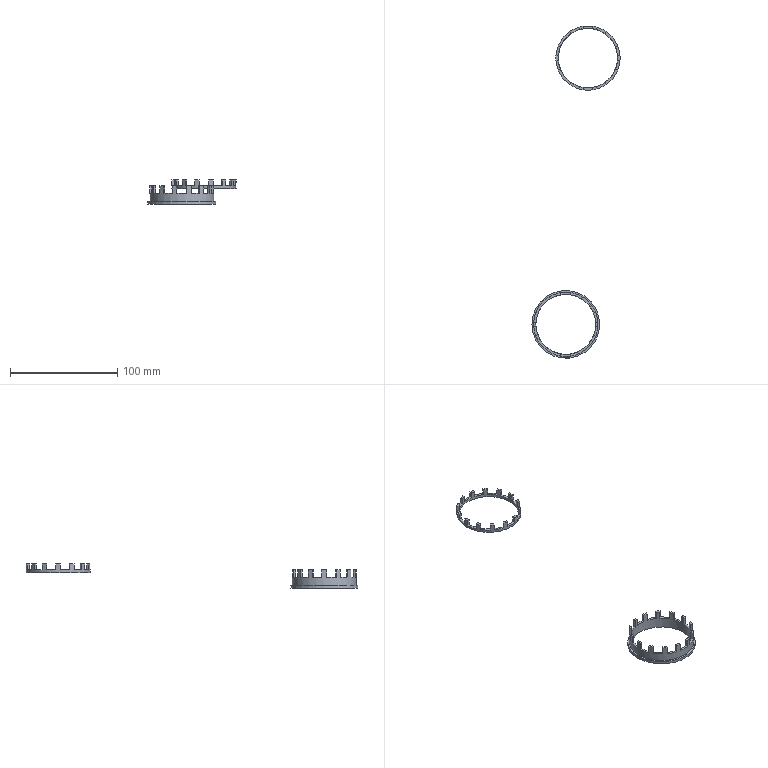NC program | NX | posted with a generic post | part box 82.344 x 310.506 x 22.5 mm
Lines 1 to 986 of 4660:
N10 G17 G21 G94 G90
(ZLEVEL_PROFILE_COPY_13_COPY_13 , TOOL : D6)
N12 T06 M6
N14 G54
N16 G17 G0 G90 X-0.856 Y-23.817 S9500 M3
N18 G43 Z30. H6
N20 Z-0.583
N22 G41 G94 G1 X-0.95 Y-23.851 F1000. D6
N24 X-1.203 Y-23.998
N26 G3 X-1.503 Y-24.518 R0.6
N28 G1 X-1.5 Y-27.736 F2200.
N30 Y-29.337
N32 X-1.501 Y-29.681
N34 Y-32.822
N36 G3 X-1.201 Y-33.341 R0.6
N38 G1 X-0.956 Y-33.483
N40 G40
N42 X-0.862 Y-33.517
N44 X0.868 Y-33.552
N46 G41 X0.962 Y-33.517 F1000.
N48 X1.201 Y-33.379
N50 G3 X1.501 Y-32.859 R0.6
N52 G1 X1.5 Y-29.337 F2200.
N54 Y-27.736
N56 X1.503 Y-24.518
N58 G3 X1.204 Y-23.998 R0.6
N60 G1 X0.95 Y-23.851
N62 G40
N64 X0.856 Y-23.817
N66 G0 X-0.855 Z-1.167
N68 G41 G1 X-0.949 Y-23.851 F1000.
N70 X-1.203 Y-23.998
N72 G3 X-1.503 Y-24.518 R0.6
N74 G1 X-1.5 Y-27.736 F2200.
N76 Y-29.337
N78 X-1.501 Y-29.681
N80 Y-32.822
N82 G3 X-1.201 Y-33.341 R0.6
N84 G1 X-0.955 Y-33.483
N86 G40
N88 X-0.862 Y-33.517
N90 X0.868 Y-33.551
N92 G41 X0.962 Y-33.517 F1000.
N94 X1.201 Y-33.379
N96 G3 X1.501 Y-32.859 R0.6
N98 G1 X1.5 Y-29.337 F2200.
N100 Y-27.736
N102 X1.503 Y-24.518
N104 G3 X1.204 Y-23.998 R0.6
N106 G1 X0.95 Y-23.851
N108 G40
N110 X0.856 Y-23.817
N112 G0 X-0.855 Z-1.75
N114 G41 G1 X-0.949 Y-23.851 F1000.
N116 X-1.203 Y-23.998
N118 G3 X-1.503 Y-24.518 R0.6
N120 G1 X-1.5 Y-27.736 F2200.
N122 Y-29.337
N124 X-1.501 Y-29.681
N126 Y-32.822
N128 G3 X-1.201 Y-33.341 R0.6
N130 G1 X-0.955 Y-33.483
N132 G40
N134 X-0.861 Y-33.517
N136 X0.868 Y-33.551
N138 G41 X0.962 Y-33.517 F1000.
N140 X1.201 Y-33.379
N142 G3 X1.501 Y-32.859 R0.6
N144 G1 X1.5 Y-29.337 F2200.
N146 Y-27.736
N148 X1.503 Y-24.518
N150 G3 X1.204 Y-23.998 R0.6
N152 G1 X0.95 Y-23.851
N154 G40
N156 X0.856 Y-23.817
N158 G0 X-0.855 Z-2.333
N160 G41 G1 X-0.949 Y-23.851 F1000.
N162 X-1.203 Y-23.998
N164 G3 X-1.502 Y-24.518 R0.6
N166 G1 X-1.5 Y-27.736 F2200.
N168 Y-29.337
N170 X-1.501 Y-29.681
N172 Y-32.822
N174 G3 X-1.201 Y-33.341 R0.6
N176 G1 X-0.955 Y-33.483
N178 G40
N180 X-0.861 Y-33.517
N182 X0.868 Y-33.551
N184 G41 X0.962 Y-33.517 F1000.
N186 X1.201 Y-33.379
N188 G3 X1.501 Y-32.859 R0.6
N190 G1 X1.5 Y-29.337 F2200.
N192 Y-27.736
N194 X1.503 Y-24.518
N196 G3 X1.204 Y-23.998 R0.6
N198 G1 X0.95 Y-23.851
N200 G40
N202 X0.856 Y-23.817
N204 G0 X-0.855 Z-2.917
N206 G41 G1 X-0.949 Y-23.851 F1000.
N208 X-1.203 Y-23.998
N210 G3 X-1.502 Y-24.518 R0.6
N212 G1 X-1.5 Y-27.736 F2200.
N214 Y-29.337
N216 X-1.501 Y-29.681
N218 Y-32.822
N220 G3 X-1.201 Y-33.341 R0.6
N222 G1 X-0.955 Y-33.483
N224 G40
N226 X-0.861 Y-33.517
N228 X0.868 Y-33.551
N230 G41 X0.962 Y-33.517 F1000.
N232 X1.201 Y-33.379
N234 G3 X1.501 Y-32.859 R0.6
N236 G1 X1.5 Y-29.337 F2200.
N238 Y-27.736
N240 X1.503 Y-24.518
N242 G3 X1.204 Y-23.998 R0.6
N244 G1 X0.95 Y-23.851
N246 G40
N248 X0.856 Y-23.817
N250 G0 X-0.855 Z-3.5
N252 G41 G1 X-0.949 Y-23.851 F1000.
N254 X-1.202 Y-23.998
N256 G3 X-1.502 Y-24.518 R0.6
N258 G1 X-1.5 Y-27.736 F2200.
N260 Y-29.337
N262 X-1.501 Y-32.822
N264 G3 X-1.201 Y-33.341 R0.6
N266 G1 X-0.955 Y-33.483
N268 G40
N270 X-0.861 Y-33.517
N272 X0.867 Y-33.551
N274 G41 X0.961 Y-33.517 F1000.
N276 X1.201 Y-33.379
N278 G3 X1.501 Y-32.859 R0.6
N280 G1 X1.5 Y-29.337 F2200.
N282 Y-27.736
N284 X1.503 Y-24.518
N286 G3 X1.204 Y-23.998 R0.6
N288 G1 X0.95 Y-23.851
N290 G40
N292 X0.856 Y-23.817
N294 G0 X-0.855 Z-4.083
N296 G41 G1 X-0.949 Y-23.851 F1000.
N298 X-1.202 Y-23.998
N300 G3 X-1.502 Y-24.518 R0.6
N302 G1 X-1.5 Y-27.736 F2200.
N304 Y-29.337
N306 X-1.501 Y-32.822
N308 G3 X-1.201 Y-33.341 R0.6
N310 G1 X-0.955 Y-33.483
N312 G40
N314 X-0.861 Y-33.517
N316 X0.867 Y-33.551
N318 G41 X0.961 Y-33.517 F1000.
N320 X1.201 Y-33.379
N322 G3 X1.501 Y-32.859 R0.6
N324 G1 X1.5 Y-29.337 F2200.
N326 Y-27.736
N328 X1.503 Y-24.518
N330 G3 X1.203 Y-23.998 R0.6
N332 G1 X0.95 Y-23.851
N334 G40
N336 X0.856 Y-23.817
N338 G0 X-0.854 Z-4.667
N340 G41 G1 X-0.948 Y-23.851 F1000.
N342 X-1.202 Y-23.998
N344 G3 X-1.502 Y-24.518 R0.6
N346 G1 X-1.5 Y-27.736 F2200.
N348 Y-29.337
N350 Y-32.822
N352 G3 X-1.2 Y-33.341 R0.6
N354 G1 X-0.955 Y-33.483
N356 G40
N358 X-0.861 Y-33.517
N360 X0.867 Y-33.551
N362 G41 X0.961 Y-33.517 F1000.
N364 X1.2 Y-33.379
N366 G3 X1.5 Y-32.859 R0.6
N368 G1 Y-29.337 F2200.
N370 Y-27.736
N372 X1.503 Y-24.518
N374 G3 X1.203 Y-23.998 R0.6
N376 G1 X0.95 Y-23.851
N378 G40
N380 X0.856 Y-23.817
N382 G0 X-0.854 Z-5.25
N384 G41 G1 X-0.948 Y-23.851 F1000.
N386 X-1.202 Y-23.998
N388 G3 X-1.502 Y-24.518 R0.6
N390 G1 X-1.5 Y-27.736 F2200.
N392 Y-29.337
N394 Y-32.822
N396 G3 X-1.2 Y-33.341 R0.6
N398 G1 X-0.955 Y-33.483
N400 G40
N402 X-0.861 Y-33.517
N404 X0.867 Y-33.551
N406 G41 X0.961 Y-33.517 F1000.
N408 X1.2 Y-33.379
N410 G3 X1.5 Y-32.859 R0.6
N412 G1 Y-29.337 F2200.
N414 Y-27.736
N416 X1.503 Y-24.518
N418 G3 X1.203 Y-23.998 R0.6
N420 G1 X0.95 Y-23.851
N422 G40
N424 X0.856 Y-23.817
N426 G0 X-0.854 Z-5.833
N428 G41 G1 X-0.948 Y-23.851 F1000.
N430 X-1.202 Y-23.998
N432 G3 X-1.501 Y-24.518 R0.6
N434 G1 X-1.5 Y-27.736 F2200.
N436 Y-29.337
N438 Y-32.822
N440 G3 X-1.2 Y-33.341 R0.6
N442 G1 X-0.955 Y-33.483
N444 G40
N446 X-0.861 Y-33.517
N448 X0.866 Y-33.546
N450 G41 X0.96 Y-33.512 F1000.
N452 X1.2 Y-33.374
N454 G3 X1.5 Y-32.854 R0.6
N456 G1 Y-29.337 F2200.
N458 Y-27.736
N460 X1.503 Y-24.518
N462 G3 X1.203 Y-23.998 R0.6
N464 G1 X0.95 Y-23.851
N466 G40
N468 X0.856 Y-23.817
N470 G0 X-0.854 Z-6.417
N472 G41 G1 X-0.948 Y-23.851 F1000.
N474 X-1.201 Y-23.998
N476 G3 X-1.501 Y-24.518 R0.6
N478 G1 X-1.5 Y-27.736 F2200.
N480 Y-29.337
N482 Y-32.822
N484 G3 X-1.2 Y-33.341 R0.6
N486 G1 X-0.955 Y-33.483
N488 G40
N490 X-0.861 Y-33.517
N492 X0.866 Y-33.546
N494 G41 X0.96 Y-33.512 F1000.
N496 X1.2 Y-33.374
N498 G3 X1.5 Y-32.854 R0.6
N500 G1 Y-29.337 F2200.
N502 Y-27.736
N504 X1.503 Y-24.518
N506 G3 X1.203 Y-23.998 R0.6
N508 G1 X0.949 Y-23.851
N510 G40
N512 X0.855 Y-23.817
N514 G0 X-0.854 Z-7.
N516 G41 G1 X-0.948 Y-23.851 F1000.
N518 X-1.201 Y-23.998
N520 G3 X-1.501 Y-24.518 R0.6
N522 G1 X-1.5 Y-27.736 F2200.
N524 Y-29.337
N526 Y-32.822
N528 G3 X-1.2 Y-33.341 R0.6
N530 G1 X-0.954 Y-33.483
N532 G40
N534 X-0.86 Y-33.517
N536 X0.866 Y-33.546
N538 G41 X0.96 Y-33.512 F1000.
N540 X1.2 Y-33.374
N542 G3 X1.5 Y-32.854 R0.6
N544 G1 Y-29.337 F2200.
N546 Y-27.736
N548 X1.503 Y-24.518
N550 G3 X1.203 Y-23.998 R0.6
N552 G1 X0.949 Y-23.851
N554 G40
N556 X0.855 Y-23.817
N558 G0 Z30.
(ZLEVEL_PROFILE_COPY_13_COPY_13_COPY , TOOL : D6)
N560 X9.563 Y-21.829
N562 Z-0.583
N564 G41 G1 X9.493 Y-21.901 F1000.
N566 X9.328 Y-22.143
N568 G3 X9.284 Y-22.742 R0.6
N570 G1 X10.683 Y-25.64 F2200.
N572 X11.377 Y-27.082
N574 X11.525 Y-27.393
N576 X12.888 Y-30.223
N578 G3 X13.384 Y-30.561 R0.6
N580 G1 X13.667 Y-30.582
N582 G40
N584 X13.766 Y-30.572
N586 X15.34 Y-29.852
N588 G41 X15.409 Y-29.781 F1000.
N590 X15.565 Y-29.552
N592 G3 X15.61 Y-28.954 R0.6
N594 G1 X14.08 Y-25.78 F2200.
N596 X13.386 Y-24.338
N598 X11.992 Y-21.437
N600 G3 X11.497 Y-21.099 R0.6
N602 G1 X11.205 Y-21.077
N604 G40
N606 X11.105 Y-21.086
N608 G0 X9.563 Y-21.829 Z-1.167
N610 G41 G1 X9.493 Y-21.901 F1000.
N612 X9.328 Y-22.143
N614 G3 X9.284 Y-22.742 R0.6
N616 G1 X10.683 Y-25.64 F2200.
N618 X11.377 Y-27.082
N620 X11.526 Y-27.393
N622 X12.888 Y-30.223
N624 G3 X13.384 Y-30.56 R0.6
N626 G1 X13.667 Y-30.582
N628 G40
N630 X13.766 Y-30.572
N632 X15.339 Y-29.852
N634 G41 X15.409 Y-29.781 F1000.
N636 X15.565 Y-29.552
N638 G3 X15.61 Y-28.954 R0.6
N640 G1 X14.08 Y-25.78 F2200.
N642 X13.386 Y-24.338
N644 X11.992 Y-21.437
N646 G3 X11.497 Y-21.099 R0.6
N648 G1 X11.205 Y-21.077
N650 G40
N652 X11.105 Y-21.087
N654 G0 X9.563 Y-21.829 Z-1.75
N656 G41 G1 X9.493 Y-21.901 F1000.
N658 X9.328 Y-22.143
N660 G3 X9.284 Y-22.742 R0.6
N662 G1 X10.683 Y-25.64 F2200.
N664 X11.377 Y-27.082
N666 X11.526 Y-27.393
N668 X12.888 Y-30.222
N670 G3 X13.384 Y-30.56 R0.6
N672 G1 X13.667 Y-30.582
N674 G40
N676 X13.766 Y-30.572
N678 X15.339 Y-29.852
N680 G41 X15.409 Y-29.781 F1000.
N682 X15.565 Y-29.552
N684 G3 X15.609 Y-28.954 R0.6
N686 G1 X14.08 Y-25.78 F2200.
N688 X13.386 Y-24.338
N690 X11.992 Y-21.437
N692 G3 X11.497 Y-21.099 R0.6
N694 G1 X11.205 Y-21.077
N696 G40
N698 X11.105 Y-21.087
N700 G0 X9.563 Y-21.829 Z-2.333
N702 G41 G1 X9.494 Y-21.901 F1000.
N704 X9.329 Y-22.143
N706 G3 X9.284 Y-22.742 R0.6
N708 G1 X10.683 Y-25.64 F2200.
N710 X11.377 Y-27.082
N712 X11.526 Y-27.393
N714 X12.889 Y-30.222
N716 G3 X13.384 Y-30.56 R0.6
N718 G1 X13.667 Y-30.582
N720 G40
N722 X13.767 Y-30.572
N724 X15.339 Y-29.852
N726 G41 X15.409 Y-29.781 F1000.
N728 X15.565 Y-29.552
N730 G3 X15.609 Y-28.954 R0.6
N732 G1 X14.08 Y-25.78 F2200.
N734 X13.386 Y-24.338
N736 X11.992 Y-21.437
N738 G3 X11.497 Y-21.099 R0.6
N740 G1 X11.204 Y-21.077
N742 G40
N744 X11.105 Y-21.087
N746 G0 X9.564 Y-21.829 Z-2.917
N748 G41 G1 X9.494 Y-21.901 F1000.
N750 X9.329 Y-22.143
N752 G3 X9.284 Y-22.741 R0.6
N754 G1 X10.683 Y-25.64 F2200.
N756 X11.377 Y-27.082
N758 X11.526 Y-27.393
N760 X12.889 Y-30.222
N762 G3 X13.384 Y-30.56 R0.6
N764 G1 X13.667 Y-30.582
N766 G40
N768 X13.767 Y-30.572
N770 X15.339 Y-29.852
N772 G41 X15.409 Y-29.781 F1000.
N774 X15.565 Y-29.552
N776 G3 X15.609 Y-28.954 R0.6
N778 G1 X14.08 Y-25.78 F2200.
N780 X13.386 Y-24.338
N782 X11.992 Y-21.438
N784 G3 X11.497 Y-21.099 R0.6
N786 G1 X11.204 Y-21.077
N788 G40
N790 X11.105 Y-21.087
N792 G0 X9.564 Y-21.829 Z-3.5
N794 G41 G1 X9.494 Y-21.901 F1000.
N796 X9.329 Y-22.143
N798 G3 X9.285 Y-22.741 R0.6
N800 G1 X10.683 Y-25.64 F2200.
N802 X11.377 Y-27.082
N804 X12.889 Y-30.222
N806 G3 X13.384 Y-30.56 R0.6
N808 G1 X13.667 Y-30.582
N810 G40
N812 X13.767 Y-30.572
N814 X15.339 Y-29.852
N816 G41 X15.409 Y-29.781 F1000.
N818 X15.564 Y-29.552
N820 G3 X15.609 Y-28.954 R0.6
N822 G1 X14.08 Y-25.78 F2200.
N824 X13.386 Y-24.338
N826 X11.992 Y-21.438
N828 G3 X11.497 Y-21.099 R0.6
N830 G1 X11.204 Y-21.077
N832 G40
N834 X11.105 Y-21.087
N836 G0 X9.564 Y-21.829 Z-4.083
N838 G41 G1 X9.494 Y-21.901 F1000.
N840 X9.329 Y-22.143
N842 G3 X9.285 Y-22.741 R0.6
N844 G1 X10.683 Y-25.64 F2200.
N846 X11.377 Y-27.082
N848 X12.889 Y-30.222
N850 G3 X13.385 Y-30.56 R0.6
N852 G1 X13.667 Y-30.582
N854 G40
N856 X13.767 Y-30.572
N858 X15.339 Y-29.852
N860 G41 X15.409 Y-29.781 F1000.
N862 X15.564 Y-29.552
N864 G3 X15.609 Y-28.954 R0.6
N866 G1 X14.08 Y-25.78 F2200.
N868 X13.386 Y-24.338
N870 X11.992 Y-21.438
N872 G3 X11.497 Y-21.099 R0.6
N874 G1 X11.204 Y-21.077
N876 G40
N878 X11.105 Y-21.087
N880 G0 X9.564 Y-21.829 Z-4.667
N882 G41 G1 X9.494 Y-21.901 F1000.
N884 X9.329 Y-22.143
N886 G3 X9.285 Y-22.741 R0.6
N888 G1 X10.683 Y-25.64 F2200.
N890 X11.377 Y-27.082
N892 X12.889 Y-30.222
N894 G3 X13.385 Y-30.56 R0.6
N896 G1 X13.667 Y-30.582
N898 G40
N900 X13.767 Y-30.572
N902 X15.339 Y-29.852
N904 G41 X15.409 Y-29.781 F1000.
N906 X15.564 Y-29.553
N908 G3 X15.609 Y-28.954 R0.6
N910 G1 X14.08 Y-25.78 F2200.
N912 X13.386 Y-24.338
N914 X11.992 Y-21.438
N916 G3 X11.496 Y-21.099 R0.6
N918 G1 X11.204 Y-21.077
N920 G40
N922 X11.105 Y-21.087
N924 G0 X9.564 Y-21.829 Z-5.25
N926 G41 G1 X9.494 Y-21.901 F1000.
N928 X9.329 Y-22.143
N930 G3 X9.285 Y-22.741 R0.6
N932 G1 X10.683 Y-25.64 F2200.
N934 X11.377 Y-27.082
N936 X12.889 Y-30.222
N938 G3 X13.385 Y-30.56 R0.6
N940 G1 X13.668 Y-30.581
N942 G40
N944 X13.767 Y-30.571
N946 X15.339 Y-29.852
N948 G41 X15.408 Y-29.781 F1000.
N950 X15.564 Y-29.553
N952 G3 X15.609 Y-28.954 R0.6
N954 G1 X14.08 Y-25.78 F2200.
N956 X13.386 Y-24.338
N958 X11.992 Y-21.438
N960 G3 X11.496 Y-21.099 R0.6
N962 G1 X11.204 Y-21.077
N964 G40
N966 X11.105 Y-21.087
N968 G0 X9.564 Y-21.829 Z-5.833
N970 G41 G1 X9.495 Y-21.901 F1000.
N972 X9.33 Y-22.143
N974 G3 X9.285 Y-22.741 R0.6
N976 G1 X10.683 Y-25.64 F2200.
N978 X11.377 Y-27.082
N980 X12.889 Y-30.222
N982 G3 X13.385 Y-30.56 R0.6
N984 G1 X13.668 Y-30.581
N986 G40
N988 X13.767 Y-30.571
N990 X15.336 Y-29.848
N992 G41 X15.405 Y-29.777 F1000.
N994 X15.562 Y-29.548
N996 G3 X15.606 Y-28.949 R0.6
N998 G1 X14.08 Y-25.78 F2200.
N1000 X13.386 Y-24.338
N1002 X11.992 Y-21.438
N1004 G3 X11.496 Y-21.099 R0.6
N1006 G1 X11.204 Y-21.077
N1008 G40
N1010 X11.105 Y-21.087
N1012 G0 X9.565 Y-21.829 Z-6.417
N1014 G41 G1 X9.495 Y-21.901 F1000.
N1016 X9.33 Y-22.143
N1018 G3 X9.285 Y-22.741 R0.6
N1020 G1 X10.683 Y-25.64 F2200.
N1022 X11.377 Y-27.082
N1024 X12.889 Y-30.222
N1026 G3 X13.385 Y-30.56 R0.6
N1028 G1 X13.668 Y-30.581
N1030 G40
N1032 X13.767 Y-30.571
N1034 X15.335 Y-29.848
N1036 G41 X15.405 Y-29.777 F1000.
N1038 X15.561 Y-29.548
N1040 G3 X15.606 Y-28.95 R0.6
N1042 G1 X14.08 Y-25.78 F2200.
N1044 X13.386 Y-24.338
N1046 X11.992 Y-21.438
N1048 G3 X11.496 Y-21.099 R0.6
N1050 G1 X11.204 Y-21.077
N1052 G40
N1054 X11.104 Y-21.087
N1056 G0 X9.565 Y-21.829 Z-7.
N1058 G41 G1 X9.495 Y-21.901 F1000.
N1060 X9.33 Y-22.143
N1062 G3 X9.285 Y-22.741 R0.6
N1064 G1 X10.683 Y-25.64 F2200.
N1066 X11.377 Y-27.082
N1068 X12.889 Y-30.222
N1070 G3 X13.385 Y-30.56 R0.6
N1072 G1 X13.668 Y-30.581
N1074 G40
N1076 X13.767 Y-30.571
N1078 X15.335 Y-29.848
N1080 G41 X15.405 Y-29.777 F1000.
N1082 X15.561 Y-29.548
N1084 G3 X15.606 Y-28.95 R0.6
N1086 G1 X14.08 Y-25.78 F2200.
N1088 X13.386 Y-24.338
N1090 X11.992 Y-21.438
N1092 G3 X11.496 Y-21.099 R0.6
N1094 G1 X11.204 Y-21.077
N1096 G40
N1098 X11.104 Y-21.087
N1100 G0 Z30.
(ZLEVEL_PROFILE_COPY_13_COPY_13_COPY_1 , TOOL : D6)
N1102 X18.087 Y-15.518
N1104 Z-0.583
N1106 G41 G1 X18.055 Y-15.613 F1000.
N1108 X18.012 Y-15.903
N1110 G3 X18.232 Y-16.462 R0.6
N1112 G1 X20.75 Y-18.466 F2200.
N1114 X22.001 Y-19.464
N1116 X22.269 Y-19.679
N1118 X24.725 Y-21.638
N1120 G3 X25.318 Y-21.727 R0.6
N1122 G1 X25.582 Y-21.623
N1124 G40
N1126 X25.668 Y-21.571
N1128 X26.773 Y-20.24
N1130 G41 X26.805 Y-20.146 F1000.
N1132 X26.846 Y-19.872
N1134 G3 X26.626 Y-19.314 R0.6
N1136 G1 X23.871 Y-17.118 F2200.
N1138 X22.62 Y-16.12
N1140 X20.106 Y-14.111
N1142 G3 X19.513 Y-14.021 R0.6
N1144 G1 X19.24 Y-14.128
N1146 G40
N1148 X19.154 Y-14.18
N1150 G0 X18.087 Y-15.518 Z-1.167
N1152 G41 G1 X18.056 Y-15.613 F1000.
N1154 X18.012 Y-15.903
N1156 G3 X18.232 Y-16.461 R0.6
N1158 G1 X20.75 Y-18.466 F2200.
N1160 X22.001 Y-19.464
N1162 X22.269 Y-19.679
N1164 X24.725 Y-21.637
N1166 G3 X25.318 Y-21.727 R0.6
N1168 G1 X25.582 Y-21.623
N1170 G40
N1172 X25.668 Y-21.571
N1174 X26.773 Y-20.24
N1176 G41 X26.805 Y-20.146 F1000.
N1178 X26.846 Y-19.872
N1180 G3 X26.626 Y-19.314 R0.6
N1182 G1 X23.871 Y-17.118 F2200.
N1184 X22.62 Y-16.12
N1186 X20.106 Y-14.111
N1188 G3 X19.513 Y-14.021 R0.6
N1190 G1 X19.24 Y-14.128
N1192 G40
N1194 X19.154 Y-14.18
N1196 G0 X18.087 Y-15.518 Z-1.75
N1198 G41 G1 X18.056 Y-15.613 F1000.
N1200 X18.012 Y-15.903
N1202 G3 X18.232 Y-16.461 R0.6
N1204 G1 X20.75 Y-18.466 F2200.
N1206 X22.001 Y-19.464
N1208 X22.269 Y-19.679
N1210 X24.725 Y-21.637
N1212 G3 X25.318 Y-21.727 R0.6
N1214 G1 X25.582 Y-21.623
N1216 G40
N1218 X25.668 Y-21.571
N1220 X26.773 Y-20.24
N1222 G41 X26.804 Y-20.146 F1000.
N1224 X26.846 Y-19.872
N1226 G3 X26.626 Y-19.314 R0.6
N1228 G1 X23.871 Y-17.118 F2200.
N1230 X22.62 Y-16.12
N1232 X20.106 Y-14.111
N1234 G3 X19.513 Y-14.021 R0.6
N1236 G1 X19.24 Y-14.128
N1238 G40
N1240 X19.154 Y-14.18
N1242 G0 X18.088 Y-15.518 Z-2.333
N1244 G41 G1 X18.056 Y-15.613 F1000.
N1246 X18.012 Y-15.903
N1248 G3 X18.232 Y-16.461 R0.6
N1250 G1 X20.75 Y-18.466 F2200.
N1252 X22.001 Y-19.464
N1254 X22.27 Y-19.679
N1256 X24.725 Y-21.637
N1258 G3 X25.318 Y-21.727 R0.6
N1260 G1 X25.582 Y-21.623
N1262 G40
N1264 X25.668 Y-21.571
N1266 X26.773 Y-20.241
N1268 G41 X26.804 Y-20.146 F1000.
N1270 X26.846 Y-19.872
N1272 G3 X26.626 Y-19.314 R0.6
N1274 G1 X23.871 Y-17.118 F2200.
N1276 X22.62 Y-16.12
N1278 X20.106 Y-14.111
N1280 G3 X19.513 Y-14.021 R0.6
N1282 G1 X19.24 Y-14.128
N1284 G40
N1286 X19.154 Y-14.18
N1288 G0 X18.088 Y-15.518 Z-2.917
N1290 G41 G1 X18.056 Y-15.613 F1000.
N1292 X18.012 Y-15.903
N1294 G3 X18.232 Y-16.461 R0.6
N1296 G1 X20.75 Y-18.466 F2200.
N1298 X22.001 Y-19.464
N1300 X22.27 Y-19.679
N1302 X24.725 Y-21.637
N1304 G3 X25.319 Y-21.727 R0.6
N1306 G1 X25.583 Y-21.623
N1308 G40
N1310 X25.668 Y-21.571
N1312 X26.772 Y-20.241
N1314 G41 X26.804 Y-20.146 F1000.
N1316 X26.845 Y-19.873
N1318 G3 X26.626 Y-19.314 R0.6
N1320 G1 X23.871 Y-17.118 F2200.
N1322 X22.62 Y-16.12
N1324 X20.106 Y-14.111
N1326 G3 X19.513 Y-14.021 R0.6
N1328 G1 X19.24 Y-14.128
N1330 G40
N1332 X19.154 Y-14.18
N1334 G0 X18.088 Y-15.518 Z-3.5
N1336 G41 G1 X18.056 Y-15.613 F1000.
N1338 X18.013 Y-15.902
N1340 G3 X18.232 Y-16.461 R0.6
N1342 G1 X20.75 Y-18.466 F2200.
N1344 X22.001 Y-19.464
N1346 X24.725 Y-21.637
N1348 G3 X25.319 Y-21.727 R0.6
N1350 G1 X25.583 Y-21.623
N1352 G40
N1354 X25.668 Y-21.571
N1356 X26.772 Y-20.241
N1358 G41 X26.804 Y-20.146 F1000.
N1360 X26.845 Y-19.873
N1362 G3 X26.626 Y-19.314 R0.6
N1364 G1 X23.871 Y-17.118 F2200.
N1366 X22.62 Y-16.12
N1368 X20.106 Y-14.111
N1370 G3 X19.513 Y-14.021 R0.6
N1372 G1 X19.24 Y-14.128
N1374 G40
N1376 X19.154 Y-14.18
N1378 G0 X18.088 Y-15.518 Z-4.083
N1380 G41 G1 X18.056 Y-15.613 F1000.
N1382 X18.013 Y-15.902
N1384 G3 X18.232 Y-16.461 R0.6
N1386 G1 X20.75 Y-18.466 F2200.
N1388 X22.001 Y-19.464
N1390 X24.725 Y-21.637
N1392 G3 X25.319 Y-21.727 R0.6
N1394 G1 X25.583 Y-21.623
N1396 G40
N1398 X25.668 Y-21.571
N1400 X26.772 Y-20.241
N1402 G41 X26.804 Y-20.146 F1000.
N1404 X26.845 Y-19.873
N1406 G3 X26.626 Y-19.314 R0.6
N1408 G1 X23.871 Y-17.118 F2200.
N1410 X22.62 Y-16.12
N1412 X20.106 Y-14.111
N1414 G3 X19.513 Y-14.021 R0.6
N1416 G1 X19.24 Y-14.128
N1418 G40
N1420 X19.154 Y-14.18
N1422 G0 X18.088 Y-15.518 Z-4.667
N1424 G41 G1 X18.056 Y-15.612 F1000.
N1426 X18.013 Y-15.902
N1428 G3 X18.232 Y-16.461 R0.6
N1430 G1 X20.75 Y-18.466 F2200.
N1432 X22.001 Y-19.464
N1434 X24.725 Y-21.637
N1436 G3 X25.319 Y-21.726 R0.6
N1438 G1 X25.583 Y-21.623
N1440 G40
N1442 X25.668 Y-21.571
N1444 X26.772 Y-20.241
N1446 G41 X26.804 Y-20.146 F1000.
N1448 X26.845 Y-19.873
N1450 G3 X26.626 Y-19.314 R0.6
N1452 G1 X23.871 Y-17.118 F2200.
N1454 X22.62 Y-16.12
N1456 X20.106 Y-14.112
N1458 G3 X19.513 Y-14.022 R0.6
N1460 G1 X19.24 Y-14.128
N1462 G40
N1464 X19.154 Y-14.18
N1466 G0 X18.088 Y-15.518 Z-5.25
N1468 G41 G1 X18.056 Y-15.612 F1000.
N1470 X18.013 Y-15.902
N1472 G3 X18.232 Y-16.46 R0.6
N1474 G1 X20.75 Y-18.466 F2200.
N1476 X22.001 Y-19.464
N1478 X24.726 Y-21.637
N1480 G3 X25.319 Y-21.726 R0.6
N1482 G1 X25.583 Y-21.623
N1484 G40
N1486 X25.668 Y-21.571
N1488 X26.772 Y-20.241
N1490 G41 X26.804 Y-20.146 F1000.
N1492 X26.845 Y-19.873
N1494 G3 X26.626 Y-19.314 R0.6
N1496 G1 X23.871 Y-17.118 F2200.
N1498 X22.62 Y-16.12
N1500 X20.106 Y-14.112
N1502 G3 X19.512 Y-14.022 R0.6
N1504 G1 X19.24 Y-14.128
N1506 G40
N1508 X19.154 Y-14.181
N1510 G0 X18.088 Y-15.517 Z-5.833
N1512 G41 G1 X18.057 Y-15.612 F1000.
N1514 X18.013 Y-15.902
N1516 G3 X18.233 Y-16.46 R0.6
N1518 G1 X20.75 Y-18.466 F2200.
N1520 X22.001 Y-19.464
N1522 X24.726 Y-21.637
N1524 G3 X25.319 Y-21.726 R0.6
N1526 G1 X25.583 Y-21.623
N1528 G40
N1530 X25.668 Y-21.571
N1532 X26.768 Y-20.239
N1534 G41 X26.799 Y-20.144 F1000.
N1536 X26.841 Y-19.87
N1538 G3 X26.622 Y-19.311 R0.6
N1540 G1 X23.871 Y-17.118 F2200.
N1542 X22.62 Y-16.12
N1544 X20.106 Y-14.112
N1546 G3 X19.512 Y-14.022 R0.6
N1548 G1 X19.24 Y-14.129
N1550 G40
N1552 X19.154 Y-14.181
N1554 G0 X18.089 Y-15.517 Z-6.417
N1556 G41 G1 X18.057 Y-15.612 F1000.
N1558 X18.013 Y-15.902
N1560 G3 X18.233 Y-16.46 R0.6
N1562 G1 X20.75 Y-18.466 F2200.
N1564 X22.001 Y-19.464
N1566 X24.726 Y-21.637
N1568 G3 X25.319 Y-21.726 R0.6
N1570 G1 X25.583 Y-21.623
N1572 G40
N1574 X25.668 Y-21.57
N1576 X26.768 Y-20.239
N1578 G41 X26.799 Y-20.144 F1000.
N1580 X26.841 Y-19.87
N1582 G3 X26.621 Y-19.311 R0.6
N1584 G1 X23.871 Y-17.118 F2200.
N1586 X22.62 Y-16.12
N1588 X20.106 Y-14.112
N1590 G3 X19.512 Y-14.022 R0.6
N1592 G1 X19.239 Y-14.129
N1594 G40
N1596 X19.154 Y-14.181
N1598 G0 X18.089 Y-15.517 Z-7.
N1600 G41 G1 X18.057 Y-15.612 F1000.
N1602 X18.013 Y-15.902
N1604 G3 X18.233 Y-16.46 R0.6
N1606 G1 X20.75 Y-18.466 F2200.
N1608 X22.001 Y-19.464
N1610 X24.726 Y-21.637
N1612 G3 X25.319 Y-21.726 R0.6
N1614 G1 X25.583 Y-21.622
N1616 G40
N1618 X25.668 Y-21.57
N1620 X26.767 Y-20.239
N1622 G41 X26.799 Y-20.144 F1000.
N1624 X26.841 Y-19.87
N1626 G3 X26.621 Y-19.311 R0.6
N1628 G1 X23.871 Y-17.118 F2200.
N1630 X22.62 Y-16.12
N1632 X20.106 Y-14.112
N1634 G3 X19.512 Y-14.022 R0.6
N1636 G1 X19.239 Y-14.129
N1638 G40
N1640 X19.154 Y-14.181
N1642 G0 Z30.
(ZLEVEL_PROFILE_COPY_13_COPY_13_COPY_2 , TOOL : D6)
N1644 X23.029 Y-6.134
N1646 Z-0.583
N1648 G41 G1 X23.042 Y-6.233 F1000.
N1650 X23.128 Y-6.513
N1652 G3 X23.569 Y-6.921 R0.6
N1654 G1 X26.707 Y-7.634 F2200.
N1656 X28.267 Y-7.99
N1658 X28.603 Y-8.068
N1660 X31.665 Y-8.767
N1662 G3 X32.238 Y-8.59 R0.6
N1664 G1 X32.431 Y-8.382
N1666 G40
N1668 X32.485 Y-8.298
N1670 X32.903 Y-6.62
N1672 G41 X32.891 Y-6.52 F1000.
N1674 X32.809 Y-6.256
N1676 G3 X32.369 Y-5.848 R0.6
N1678 G1 X28.935 Y-5.066 F2200.
N1680 X27.374 Y-4.709
N1682 X24.238 Y-3.99
N1684 G3 X23.664 Y-4.166 R0.6
N1686 G1 X23.464 Y-4.381
N1688 G40
N1690 X23.41 Y-4.465
N1692 G0 X23.029 Y-6.134 Z-1.167
N1694 G41 G1 X23.042 Y-6.233 F1000.
N1696 X23.128 Y-6.513
N1698 G3 X23.569 Y-6.921 R0.6
N1700 G1 X26.707 Y-7.634 F2200.
N1702 X28.267 Y-7.99
N1704 X28.603 Y-8.068
N1706 X31.665 Y-8.767
N1708 G3 X32.238 Y-8.59 R0.6
N1710 G1 X32.431 Y-8.382
N1712 G40
N1714 X32.485 Y-8.298
N1716 X32.903 Y-6.62
N1718 G41 X32.891 Y-6.521 F1000.
N1720 X32.809 Y-6.256
N1722 G3 X32.369 Y-5.848 R0.6
N1724 G1 X28.935 Y-5.066 F2200.
N1726 X27.374 Y-4.709
N1728 X24.238 Y-3.99
N1730 G3 X23.664 Y-4.166 R0.6
N1732 G1 X23.464 Y-4.381
N1734 G40
N1736 X23.41 Y-4.465
N1738 G0 X23.029 Y-6.134 Z-1.75
N1740 G41 G1 X23.042 Y-6.233 F1000.
N1742 X23.128 Y-6.513
N1744 G3 X23.569 Y-6.921 R0.6
N1746 G1 X26.707 Y-7.634 F2200.
N1748 X28.267 Y-7.99
N1750 X28.603 Y-8.068
N1752 X31.665 Y-8.767
N1754 G3 X32.238 Y-8.59 R0.6
N1756 G1 X32.431 Y-8.382
N1758 G40
N1760 X32.485 Y-8.298
N1762 X32.903 Y-6.62
N1764 G41 X32.891 Y-6.521 F1000.
N1766 X32.809 Y-6.257
N1768 G3 X32.369 Y-5.849 R0.6
N1770 G1 X28.935 Y-5.066 F2200.
N1772 X27.374 Y-4.709
N1774 X24.238 Y-3.99
N1776 G3 X23.664 Y-4.166 R0.6
N1778 G1 X23.464 Y-4.381
N1780 G40
N1782 X23.41 Y-4.465
N1784 G0 X23.029 Y-6.133 Z-2.333
N1786 G41 G1 X23.042 Y-6.233 F1000.
N1788 X23.129 Y-6.513
N1790 G3 X23.569 Y-6.92 R0.6
N1792 G1 X26.707 Y-7.634 F2200.
N1794 X28.267 Y-7.99
N1796 X28.603 Y-8.068
N1798 X31.665 Y-8.767
N1800 G3 X32.238 Y-8.59 R0.6
N1802 G1 X32.431 Y-8.382
N1804 G40
N1806 X32.485 Y-8.298
N1808 X32.903 Y-6.62
N1810 G41 X32.891 Y-6.521 F1000.
N1812 X32.809 Y-6.257
N1814 G3 X32.369 Y-5.849 R0.6
N1816 G1 X28.935 Y-5.066 F2200.
N1818 X27.374 Y-4.709
N1820 X24.237 Y-3.99
N1822 G3 X23.664 Y-4.166 R0.6
N1824 G1 X23.464 Y-4.381
N1826 G40
N1828 X23.41 Y-4.465
N1830 G0 X23.029 Y-6.133 Z-2.917
N1832 G41 G1 X23.042 Y-6.232 F1000.
N1834 X23.129 Y-6.512
N1836 G3 X23.569 Y-6.92 R0.6
N1838 G1 X26.707 Y-7.634 F2200.
N1840 X28.267 Y-7.99
N1842 X28.603 Y-8.068
N1844 X31.665 Y-8.767
N1846 G3 X32.238 Y-8.59 R0.6
N1848 G1 X32.431 Y-8.382
N1850 G40
N1852 X32.485 Y-8.298
N1854 X32.903 Y-6.62
N1856 G41 X32.891 Y-6.521 F1000.
N1858 X32.809 Y-6.257
N1860 G3 X32.369 Y-5.849 R0.6
N1862 G1 X28.935 Y-5.066 F2200.
N1864 X27.374 Y-4.709
N1866 X24.237 Y-3.99
N1868 G3 X23.664 Y-4.167 R0.6
N1870 G1 X23.464 Y-4.381
N1872 G40
N1874 X23.41 Y-4.465
N1876 G0 X23.03 Y-6.133 Z-3.5
N1878 G41 G1 X23.042 Y-6.232 F1000.
N1880 X23.129 Y-6.512
N1882 G3 X23.569 Y-6.92 R0.6
N1884 G1 X26.707 Y-7.634 F2200.
N1886 X28.267 Y-7.99
N1888 X31.665 Y-8.766
N1890 G3 X32.238 Y-8.59 R0.6
N1892 G1 X32.431 Y-8.382
N1894 G40
N1896 X32.485 Y-8.298
N1898 X32.903 Y-6.62
N1900 G41 X32.891 Y-6.521 F1000.
N1902 X32.809 Y-6.257
N1904 G3 X32.369 Y-5.849 R0.6
N1906 G1 X28.935 Y-5.066 F2200.
N1908 X27.374 Y-4.709
N1910 X24.237 Y-3.99
N1912 G3 X23.664 Y-4.167 R0.6
N1914 G1 X23.464 Y-4.381
N1916 G40
N1918 X23.41 Y-4.465
N1920 G0 X23.03 Y-6.133 Z-4.083
N1922 G41 G1 X23.042 Y-6.232 F1000.
N1924 X23.129 Y-6.512
N1926 G3 X23.569 Y-6.92 R0.6
N1928 G1 X26.707 Y-7.634 F2200.
N1930 X28.267 Y-7.99
N1932 X31.665 Y-8.766
N1934 G3 X32.238 Y-8.59 R0.6
N1936 G1 X32.431 Y-8.382
N1938 G40
N1940 X32.485 Y-8.298
N1942 X32.903 Y-6.62
N1944 G41 X32.891 Y-6.521 F1000.
N1946 X32.809 Y-6.257
N1948 G3 X32.369 Y-5.849 R0.6
N1950 G1 X28.935 Y-5.066 F2200.
N1952 X27.374 Y-4.709